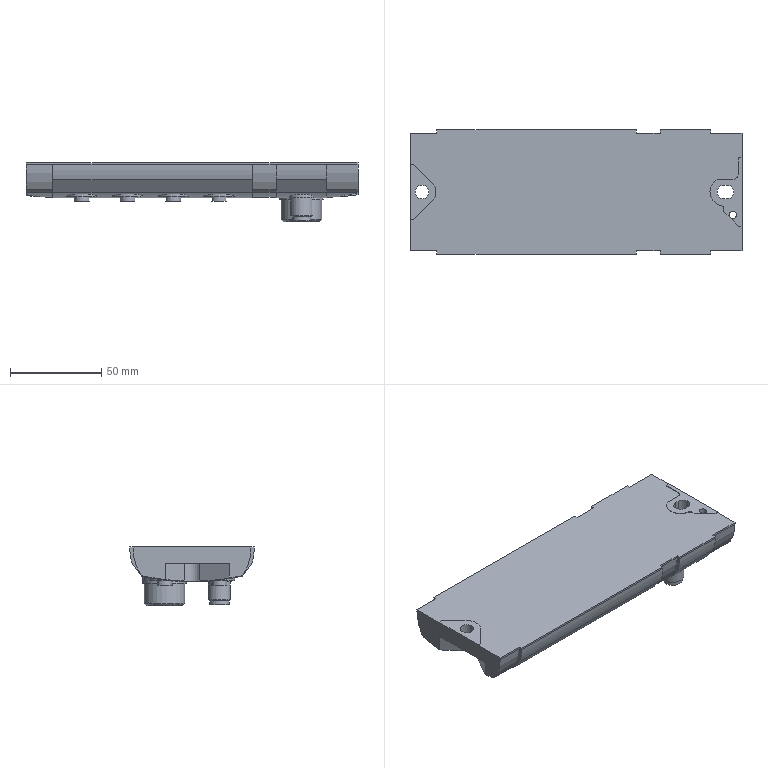Part | NX | features 5003_105_IO ring module 2 | 1 solid | 234 faces | box 181.5 x 68 x 32.4 mm | volume 204589 mm3 | plane 125 | cylinder 106 | cone 3 | commonest cylinder face diameters 1.1 x40 8.2 x8 16.6 x8 6 x7 51.4 x6 1 x4